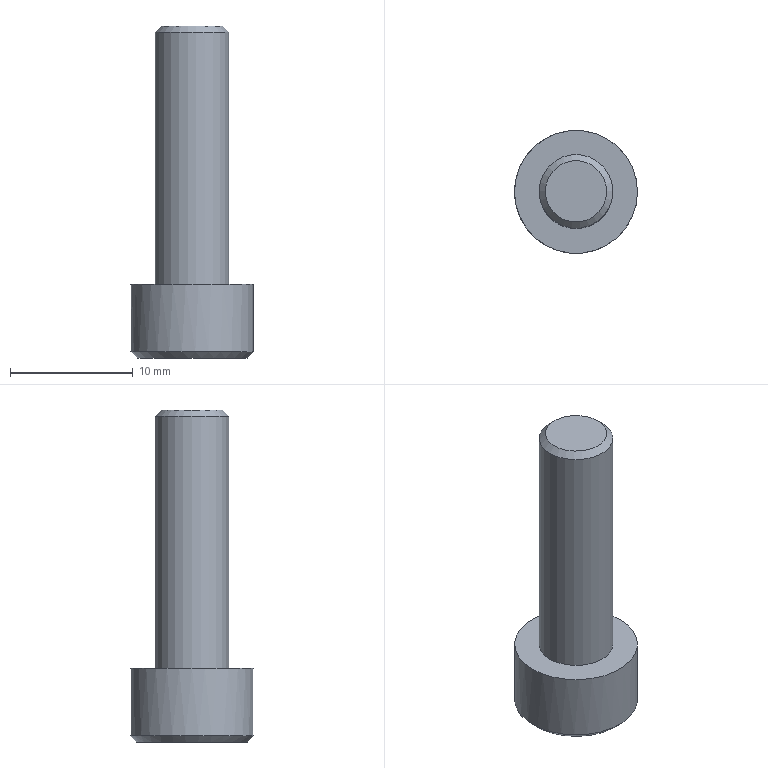Part | STEP file | gslz 2016.10.28-6_id234_x_t | 1 solid | 14 faces | box 10 x 10 x 27 mm | volume 972.376 mm3 | plane 10 | cylinder 2 | cone 2 | commonest cylinder face diameters 6 x1 10 x1
STEP:
#1=CARTESIAN_POINT('',(-2.5,155.,123.992));
#2=VERTEX_POINT('',#1);
#3=CARTESIAN_POINT('',(-7.,155.,123.992));
#4=DIRECTION('',(0.,0.,-1.));
#5=DIRECTION('',(1.,0.,0.));
#6=AXIS2_PLACEMENT_3D('',#3,#4,#5);
#7=CIRCLE('',#6,4.5);
#8=EDGE_CURVE('',#2,#2,#7,.T.);
#9=ORIENTED_EDGE('',*,*,#8,.T.);
#10=EDGE_LOOP('',(#9));
#11=FACE_BOUND('',#10,.T.);
#12=CARTESIAN_POINT('',(-9.5,153.557,123.992));
#13=VERTEX_POINT('',#12);
#14=CARTESIAN_POINT('',(-9.5,156.443,123.992));
#15=VERTEX_POINT('',#14);
#16=CARTESIAN_POINT('',(-9.5,153.557,123.992));
#17=DIRECTION('',(0.,1.,0.));
#18=VECTOR('',#17,1.);
#19=LINE('',#16,#18);
#20=EDGE_CURVE('',#13,#15,#19,.T.);
#21=ORIENTED_EDGE('',*,*,#20,.F.);
#22=CARTESIAN_POINT('',(-7.,152.113,123.992));
#23=VERTEX_POINT('',#22);
#24=CARTESIAN_POINT('',(-7.,152.113,123.992));
#25=DIRECTION('',(-0.866,0.5,0.));
#26=VECTOR('',#25,1.);
#27=LINE('',#24,#26);
#28=EDGE_CURVE('',#23,#13,#27,.T.);
#29=ORIENTED_EDGE('',*,*,#28,.F.);
#30=CARTESIAN_POINT('',(-4.5,153.557,123.992));
#31=VERTEX_POINT('',#30);
#32=CARTESIAN_POINT('',(-4.5,153.557,123.992));
#33=DIRECTION('',(-0.866,-0.5,0.));
#34=VECTOR('',#33,1.);
#35=LINE('',#32,#34);
#36=EDGE_CURVE('',#31,#23,#35,.T.);
#37=ORIENTED_EDGE('',*,*,#36,.F.);
#38=CARTESIAN_POINT('',(-4.5,156.443,123.992));
#39=VERTEX_POINT('',#38);
#40=CARTESIAN_POINT('',(-4.5,156.443,123.992));
#41=DIRECTION('',(0.,-1.,0.));
#42=VECTOR('',#41,1.);
#43=LINE('',#40,#42);
#44=EDGE_CURVE('',#39,#31,#43,.T.);
#45=ORIENTED_EDGE('',*,*,#44,.F.);
#46=CARTESIAN_POINT('',(-7.,157.887,123.992));
#47=VERTEX_POINT('',#46);
#48=CARTESIAN_POINT('',(-7.,157.887,123.992));
#49=DIRECTION('',(0.866,-0.5,0.));
#50=VECTOR('',#49,1.);
#51=LINE('',#48,#50);
#52=EDGE_CURVE('',#47,#39,#51,.T.);
#53=ORIENTED_EDGE('',*,*,#52,.F.);
#54=CARTESIAN_POINT('',(-9.5,156.443,123.992));
#55=DIRECTION('',(0.866,0.5,0.));
#56=VECTOR('',#55,1.);
#57=LINE('',#54,#56);
#58=EDGE_CURVE('',#15,#47,#57,.T.);
#59=ORIENTED_EDGE('',*,*,#58,.F.);
#60=EDGE_LOOP('',(#21,#29,#37,#45,#53,#59));
#61=FACE_BOUND('',#60,.T.);
#62=CARTESIAN_POINT('',(-7.,155.,123.992));
#63=DIRECTION('',(0.,0.,-1.));
#64=DIRECTION('',(-1.,0.,0.));
#65=AXIS2_PLACEMENT_3D('',#62,#63,#64);
#66=PLANE('',#65);
#67=ADVANCED_FACE('',(#11,#61),#66,.T.);
#68=CARTESIAN_POINT('',(-9.5,155.,150.992));
#69=VERTEX_POINT('',#68);
#70=CARTESIAN_POINT('',(-7.,155.,150.992));
#71=DIRECTION('',(0.,0.,1.));
#72=DIRECTION('',(-1.,0.,0.));
#73=AXIS2_PLACEMENT_3D('',#70,#71,#72);
#74=CIRCLE('',#73,2.5);
#75=EDGE_CURVE('',#69,#69,#74,.T.);
#76=ORIENTED_EDGE('',*,*,#75,.T.);
#77=EDGE_LOOP('',(#76));
#78=FACE_OUTER_BOUND('',#77,.T.);
#79=CARTESIAN_POINT('',(-7.,155.,150.992));
#80=DIRECTION('',(0.,0.,1.));
#81=DIRECTION('',(1.,0.,0.));
#82=AXIS2_PLACEMENT_3D('',#79,#80,#81);
#83=PLANE('',#82);
#84=ADVANCED_FACE('',(#78),#83,.T.);
#85=CARTESIAN_POINT('',(-4.,155.,150.492));
#86=VERTEX_POINT('',#85);
#87=CARTESIAN_POINT('',(-7.,155.,150.492));
#88=DIRECTION('',(0.,0.,-1.));
#89=DIRECTION('',(1.,0.,0.));
#90=AXIS2_PLACEMENT_3D('',#87,#88,#89);
#91=CIRCLE('',#90,3.);
#92=EDGE_CURVE('',#86,#86,#91,.T.);
#93=ORIENTED_EDGE('',*,*,#92,.T.);
#94=EDGE_LOOP('',(#93));
#95=FACE_BOUND('',#94,.T.);
#96=CARTESIAN_POINT('',(-10.,155.,129.992));
#97=VERTEX_POINT('',#96);
#98=CARTESIAN_POINT('',(-7.,155.,129.992));
#99=DIRECTION('',(0.,0.,1.));
#100=DIRECTION('',(-1.,0.,0.));
#101=AXIS2_PLACEMENT_3D('',#98,#99,#100);
#102=CIRCLE('',#101,3.);
#103=EDGE_CURVE('',#97,#97,#102,.T.);
#104=ORIENTED_EDGE('',*,*,#103,.T.);
#105=EDGE_LOOP('',(#104));
#106=FACE_BOUND('',#105,.T.);
#107=CARTESIAN_POINT('',(-7.,155.,141.992));
#108=DIRECTION('',(0.,0.,1.));
#109=DIRECTION('',(1.,0.,0.));
#110=AXIS2_PLACEMENT_3D('',#107,#108,#109);
#111=CYLINDRICAL_SURFACE('',#110,3.);
#112=ADVANCED_FACE('',(#95,#106),#111,.T.);
#113=ORIENTED_EDGE('',*,*,#103,.F.);
#114=EDGE_LOOP('',(#113));
#115=FACE_BOUND('',#114,.T.);
#116=CARTESIAN_POINT('',(-12.,155.,129.992));
#117=VERTEX_POINT('',#116);
#118=CARTESIAN_POINT('',(-7.,155.,129.992));
#119=DIRECTION('',(0.,0.,1.));
#120=DIRECTION('',(-1.,0.,0.));
#121=AXIS2_PLACEMENT_3D('',#118,#119,#120);
#122=CIRCLE('',#121,5.);
#123=EDGE_CURVE('',#117,#117,#122,.T.);
#124=ORIENTED_EDGE('',*,*,#123,.T.);
#125=EDGE_LOOP('',(#124));
#126=FACE_BOUND('',#125,.T.);
#127=CARTESIAN_POINT('',(-7.,155.,129.992));
#128=DIRECTION('',(0.,0.,1.));
#129=DIRECTION('',(1.,0.,0.));
#130=AXIS2_PLACEMENT_3D('',#127,#128,#129);
#131=PLANE('',#130);
#132=ADVANCED_FACE('',(#115,#126),#131,.T.);
#133=CARTESIAN_POINT('',(-2.,155.,124.492));
#134=VERTEX_POINT('',#133);
#135=CARTESIAN_POINT('',(-7.,155.,124.492));
#136=DIRECTION('',(0.,0.,1.));
#137=DIRECTION('',(1.,0.,0.));
#138=AXIS2_PLACEMENT_3D('',#135,#136,#137);
#139=CIRCLE('',#138,5.);
#140=EDGE_CURVE('',#134,#134,#139,.T.);
#141=ORIENTED_EDGE('',*,*,#140,.T.);
#142=EDGE_LOOP('',(#141));
#143=FACE_BOUND('',#142,.T.);
#144=ORIENTED_EDGE('',*,*,#123,.F.);
#145=EDGE_LOOP('',(#144));
#146=FACE_BOUND('',#145,.T.);
#147=CARTESIAN_POINT('',(-7.,155.,121.992));
#148=DIRECTION('',(0.,0.,1.));
#149=DIRECTION('',(1.,0.,0.));
#150=AXIS2_PLACEMENT_3D('',#147,#148,#149);
#151=CYLINDRICAL_SURFACE('',#150,5.);
#152=ADVANCED_FACE('',(#143,#146),#151,.T.);
#153=ORIENTED_EDGE('',*,*,#92,.F.);
#154=EDGE_LOOP('',(#153));
#155=FACE_BOUND('',#154,.T.);
#156=ORIENTED_EDGE('',*,*,#75,.F.);
#157=EDGE_LOOP('',(#156));
#158=FACE_BOUND('',#157,.T.);
#159=CARTESIAN_POINT('',(-7.,155.,150.992));
#160=DIRECTION('',(0.,0.,-1.));
#161=DIRECTION('',(1.,0.,0.));
#162=AXIS2_PLACEMENT_3D('',#159,#160,#161);
#163=CONICAL_SURFACE('',#162,2.5,45.);
#164=ADVANCED_FACE('',(#155,#158),#163,.T.);
#165=ORIENTED_EDGE('',*,*,#20,.T.);
#166=CARTESIAN_POINT('',(-9.5,156.443,127.992));
#167=VERTEX_POINT('',#166);
#168=CARTESIAN_POINT('',(-9.5,156.443,127.992));
#169=DIRECTION('',(0.,0.,1.));
#170=VECTOR('',#169,1.);
#171=LINE('',#168,#170);
#172=EDGE_CURVE('',#15,#167,#171,.T.);
#173=ORIENTED_EDGE('',*,*,#172,.T.);
#174=CARTESIAN_POINT('',(-9.5,153.557,127.992));
#175=VERTEX_POINT('',#174);
#176=CARTESIAN_POINT('',(-9.5,153.557,127.992));
#177=DIRECTION('',(0.,-1.,0.));
#178=VECTOR('',#177,1.);
#179=LINE('',#176,#178);
#180=EDGE_CURVE('',#167,#175,#179,.T.);
#181=ORIENTED_EDGE('',*,*,#180,.T.);
#182=CARTESIAN_POINT('',(-9.5,153.557,127.992));
#183=DIRECTION('',(0.,0.,1.));
#184=VECTOR('',#183,1.);
#185=LINE('',#182,#184);
#186=EDGE_CURVE('',#13,#175,#185,.T.);
#187=ORIENTED_EDGE('',*,*,#186,.F.);
#188=EDGE_LOOP('',(#165,#173,#181,#187));
#189=FACE_OUTER_BOUND('',#188,.T.);
#190=CARTESIAN_POINT('',(-9.5,153.557,127.992));
#191=DIRECTION('',(-1.,0.,0.));
#192=DIRECTION('',(0.,0.,1.));
#193=AXIS2_PLACEMENT_3D('',#190,#191,#192);
#194=PLANE('',#193);
#195=ADVANCED_FACE('',(#189),#194,.F.);
#196=ORIENTED_EDGE('',*,*,#58,.T.);
#197=CARTESIAN_POINT('',(-7.,157.887,127.992));
#198=VERTEX_POINT('',#197);
#199=CARTESIAN_POINT('',(-7.,157.887,127.992));
#200=DIRECTION('',(0.,0.,1.));
#201=VECTOR('',#200,1.);
#202=LINE('',#199,#201);
#203=EDGE_CURVE('',#47,#198,#202,.T.);
#204=ORIENTED_EDGE('',*,*,#203,.T.);
#205=CARTESIAN_POINT('',(-9.5,156.443,127.992));
#206=DIRECTION('',(-0.866,-0.5,0.));
#207=VECTOR('',#206,1.);
#208=LINE('',#205,#207);
#209=EDGE_CURVE('',#198,#167,#208,.T.);
#210=ORIENTED_EDGE('',*,*,#209,.T.);
#211=ORIENTED_EDGE('',*,*,#172,.F.);
#212=EDGE_LOOP('',(#196,#204,#210,#211));
#213=FACE_OUTER_BOUND('',#212,.T.);
#214=CARTESIAN_POINT('',(-9.5,156.443,127.992));
#215=DIRECTION('',(-0.5,0.866,0.));
#216=DIRECTION('',(-0.866,-0.5,0.));
#217=AXIS2_PLACEMENT_3D('',#214,#215,#216);
#218=PLANE('',#217);
#219=ADVANCED_FACE('',(#213),#218,.F.);
#220=ORIENTED_EDGE('',*,*,#52,.T.);
#221=CARTESIAN_POINT('',(-4.5,156.443,127.992));
#222=VERTEX_POINT('',#221);
#223=CARTESIAN_POINT('',(-4.5,156.443,127.992));
#224=DIRECTION('',(0.,0.,1.));
#225=VECTOR('',#224,1.);
#226=LINE('',#223,#225);
#227=EDGE_CURVE('',#39,#222,#226,.T.);
#228=ORIENTED_EDGE('',*,*,#227,.T.);
#229=CARTESIAN_POINT('',(-7.,157.887,127.992));
#230=DIRECTION('',(-0.866,0.5,0.));
#231=VECTOR('',#230,1.);
#232=LINE('',#229,#231);
#233=EDGE_CURVE('',#222,#198,#232,.T.);
#234=ORIENTED_EDGE('',*,*,#233,.T.);
#235=ORIENTED_EDGE('',*,*,#203,.F.);
#236=EDGE_LOOP('',(#220,#228,#234,#235));
#237=FACE_OUTER_BOUND('',#236,.T.);
#238=CARTESIAN_POINT('',(-7.,157.887,127.992));
#239=DIRECTION('',(0.5,0.866,0.));
#240=DIRECTION('',(-0.866,0.5,0.));
#241=AXIS2_PLACEMENT_3D('',#238,#239,#240);
#242=PLANE('',#241);
#243=ADVANCED_FACE('',(#237),#242,.F.);
#244=ORIENTED_EDGE('',*,*,#44,.T.);
#245=CARTESIAN_POINT('',(-4.5,153.557,127.992));
#246=VERTEX_POINT('',#245);
#247=CARTESIAN_POINT('',(-4.5,153.557,127.992));
#248=DIRECTION('',(0.,0.,1.));
#249=VECTOR('',#248,1.);
#250=LINE('',#247,#249);
#251=EDGE_CURVE('',#31,#246,#250,.T.);
#252=ORIENTED_EDGE('',*,*,#251,.T.);
#253=CARTESIAN_POINT('',(-4.5,156.443,127.992));
#254=DIRECTION('',(0.,1.,0.));
#255=VECTOR('',#254,1.);
#256=LINE('',#253,#255);
#257=EDGE_CURVE('',#246,#222,#256,.T.);
#258=ORIENTED_EDGE('',*,*,#257,.T.);
#259=ORIENTED_EDGE('',*,*,#227,.F.);
#260=EDGE_LOOP('',(#244,#252,#258,#259));
#261=FACE_OUTER_BOUND('',#260,.T.);
#262=CARTESIAN_POINT('',(-4.5,156.443,127.992));
#263=DIRECTION('',(1.,0.,0.));
#264=DIRECTION('',(0.,0.,-1.));
#265=AXIS2_PLACEMENT_3D('',#262,#263,#264);
#266=PLANE('',#265);
#267=ADVANCED_FACE('',(#261),#266,.F.);
#268=ORIENTED_EDGE('',*,*,#36,.T.);
#269=CARTESIAN_POINT('',(-7.,152.113,127.992));
#270=VERTEX_POINT('',#269);
#271=CARTESIAN_POINT('',(-7.,152.113,127.992));
#272=DIRECTION('',(0.,0.,1.));
#273=VECTOR('',#272,1.);
#274=LINE('',#271,#273);
#275=EDGE_CURVE('',#23,#270,#274,.T.);
#276=ORIENTED_EDGE('',*,*,#275,.T.);
#277=CARTESIAN_POINT('',(-4.5,153.557,127.992));
#278=DIRECTION('',(0.866,0.5,0.));
#279=VECTOR('',#278,1.);
#280=LINE('',#277,#279);
#281=EDGE_CURVE('',#270,#246,#280,.T.);
#282=ORIENTED_EDGE('',*,*,#281,.T.);
#283=ORIENTED_EDGE('',*,*,#251,.F.);
#284=EDGE_LOOP('',(#268,#276,#282,#283));
#285=FACE_OUTER_BOUND('',#284,.T.);
#286=CARTESIAN_POINT('',(-4.5,153.557,127.992));
#287=DIRECTION('',(0.5,-0.866,0.));
#288=DIRECTION('',(0.866,0.5,0.));
#289=AXIS2_PLACEMENT_3D('',#286,#287,#288);
#290=PLANE('',#289);
#291=ADVANCED_FACE('',(#285),#290,.F.);
#292=ORIENTED_EDGE('',*,*,#28,.T.);
#293=ORIENTED_EDGE('',*,*,#186,.T.);
#294=CARTESIAN_POINT('',(-7.,152.113,127.992));
#295=DIRECTION('',(0.866,-0.5,0.));
#296=VECTOR('',#295,1.);
#297=LINE('',#294,#296);
#298=EDGE_CURVE('',#175,#270,#297,.T.);
#299=ORIENTED_EDGE('',*,*,#298,.T.);
#300=ORIENTED_EDGE('',*,*,#275,.F.);
#301=EDGE_LOOP('',(#292,#293,#299,#300));
#302=FACE_OUTER_BOUND('',#301,.T.);
#303=CARTESIAN_POINT('',(-7.,152.113,127.992));
#304=DIRECTION('',(-0.5,-0.866,0.));
#305=DIRECTION('',(0.866,-0.5,0.));
#306=AXIS2_PLACEMENT_3D('',#303,#304,#305);
#307=PLANE('',#306);
#308=ADVANCED_FACE('',(#302),#307,.F.);
#309=ORIENTED_EDGE('',*,*,#180,.F.);
#310=ORIENTED_EDGE('',*,*,#209,.F.);
#311=ORIENTED_EDGE('',*,*,#233,.F.);
#312=ORIENTED_EDGE('',*,*,#257,.F.);
#313=ORIENTED_EDGE('',*,*,#281,.F.);
#314=ORIENTED_EDGE('',*,*,#298,.F.);
#315=EDGE_LOOP('',(#309,#310,#311,#312,#313,#314));
#316=FACE_OUTER_BOUND('',#315,.T.);
#317=CARTESIAN_POINT('',(-9.5,156.443,127.992));
#318=DIRECTION('',(0.,0.,-1.));
#319=DIRECTION('',(-1.,0.,0.));
#320=AXIS2_PLACEMENT_3D('',#317,#318,#319);
#321=PLANE('',#320);
#322=ADVANCED_FACE('',(#316),#321,.T.);
#323=ORIENTED_EDGE('',*,*,#8,.F.);
#324=EDGE_LOOP('',(#323));
#325=FACE_BOUND('',#324,.T.);
#326=ORIENTED_EDGE('',*,*,#140,.F.);
#327=EDGE_LOOP('',(#326));
#328=FACE_BOUND('',#327,.T.);
#329=CARTESIAN_POINT('',(-7.,155.,124.492));
#330=DIRECTION('',(0.,0.,1.));
#331=DIRECTION('',(1.,0.,0.));
#332=AXIS2_PLACEMENT_3D('',#329,#330,#331);
#333=CONICAL_SURFACE('',#332,5.,45.);
#334=ADVANCED_FACE('',(#325,#328),#333,.T.);
#335=CLOSED_SHELL('',(#67,#84,#112,#132,#152,#164,#195,#219,#243,#267,#291,#308,#322,#334));
#336=MANIFOLD_SOLID_BREP('',#335);
#337=(LENGTH_UNIT()NAMED_UNIT(*)SI_UNIT(.MILLI.,.METRE.));
#338=UNCERTAINTY_MEASURE_WITH_UNIT(LENGTH_MEASURE(0.00002),#337,'','');
#339=(NAMED_UNIT(*)PLANE_ANGLE_UNIT()SI_UNIT($,.RADIAN.));
#340=PLANE_ANGLE_MEASURE_WITH_UNIT(PLANE_ANGLE_MEASURE(0.01745),#339);
#341=DIMENSIONAL_EXPONENTS(0.,0.,0.,0.,0.,0.,0.);
#342=(CONVERSION_BASED_UNIT('DEGREE',#340)NAMED_UNIT(#341)PLANE_ANGLE_UNIT());
#343=(NAMED_UNIT(*)SI_UNIT($,.STERADIAN.)SOLID_ANGLE_UNIT());
#344=(GEOMETRIC_REPRESENTATION_CONTEXT(3)GLOBAL_UNCERTAINTY_ASSIGNED_CONTEXT((#338))GLOBAL_UNIT_ASSIGNED_CONTEXT((#337,#342,#343))REPRESENTATION_CONTEXT('',''));
#345=ADVANCED_BREP_SHAPE_REPRESENTATION('',(#336),#344);